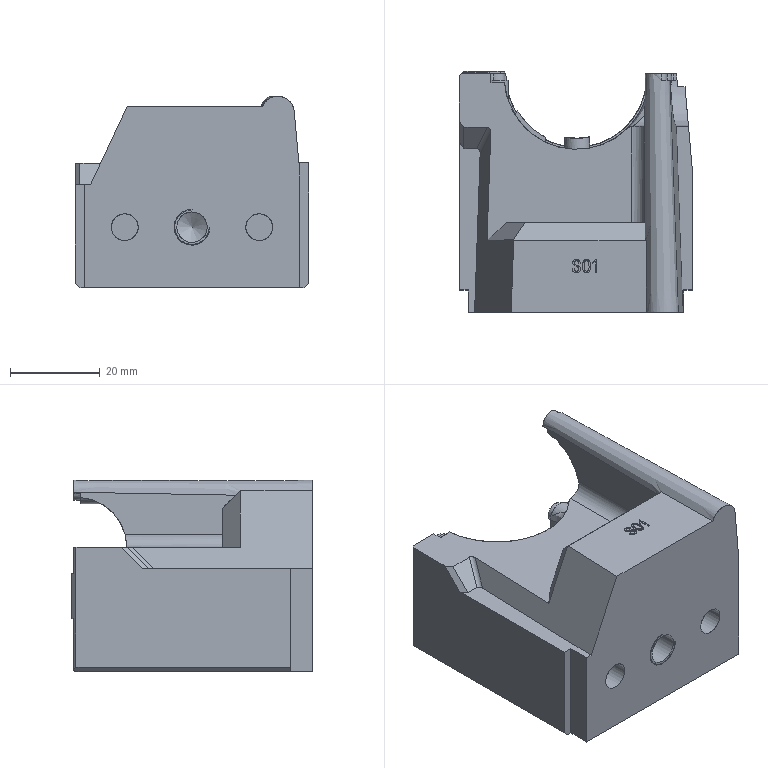NC program | PowerMill | posted with a generic post | part box 52 x 53.756 x 42.711 mm
Lines 1 to 909 of 52163:
%
O0001
N104 ( POWERMILL CB  : 2026004.0)
N105 ( POST VER      : 2026.0.0.5161)
N106 ( OPTION FILE   : FANUC)
N107 ( OUTPUT WORKPLANE : 2)
N108 (  )
N109 ( TOOL LIST )
N110 (---------------------------------------)
N111 ( NO. | ID        | DIA.| TIP RAD|LENGTH)
N112 (---------------------------------------)
N113 (    1|B13R0.8_1_1|13.0 |  0.8   |116.16)
N114 (---------------------------------------)
N115 (  )
N116 ( NUMBER OF TOOLPATHS: 1.0 )
N117 ( ESTIMATED PROGRAM DURATION: 0 HOURS 17 MIN 51 SEC)
N118 (  )
N119 G00 G21 G80 G40 G17
N120 G90
N121 G54
N122 G53 Z0.0
N123 (---------------)
N124 ( START TOOLPATH : 05开粗-B13R0.8-偏置区域清除 )
N125 (---------------)
N126 ( TOOL NO.    :1 )
N127 ( TOOL TYPE   : TIPRADIUSED)
N128 ( TOOL ID     : B13R0.8_1_1)
N129 ( TOOL DIA    : 13.0 LENGTH 116.16)
N130 T1
N131 M6
N132 S2200 M03
N133 G00 G90 X0.1113 Y-6.4944
N134 G43 Z74.256 H1
N135
N136 G05 P10000 R8
N137 Z57.1261
N138 G01 Z54.1261 F2400.0
N139 X0.1108 Y-6.1369 F4000.0
N140 X0.0999 Y0.7514
N141 X0.0891 Y7.6396
N142 X0.0782 Y14.5279
N143 X0.0675 Y21.3365
N144 X4.0078 Y21.3427
N145 G03 X4.3816 Y21.7172 I-0.0006 J0.3745
N146 G01 Y21.9928
N147 G03 X4.0078 Y22.3673 I-0.3744 J0.0
N148 G01 X-3.8728 Y22.3797
N149 G03 X-4.2726 Y21.9805 I-0.0006 J-0.3992
N150 G01 Y21.7295
N151 G03 X-3.8728 Y21.3303 I0.3992 J0.0
N152 G01 X0.0675 Y21.3365
N153 X0.0782 Y14.5279
N154 X9.1921
N155 G03 X11.4721 Y16.8079 I0.0 J2.28
N156 G01 Y26.9021
N157 G03 X9.1921 Y29.1821 I-2.28 J0.0
N158 G01 X-9.1921
N159 G03 X-11.4721 Y26.9021 I0.0 J-2.28
N160 G01 Y16.8079
N161 G03 X-9.1921 Y14.5279 I2.28 J0.0
N162 G01 X0.0782
N163 X0.0891 Y7.6396
N164 X16.0804
N165 G03 X18.3604 Y9.9196 I0.0 J2.28
N166 G01 Y33.7904
N167 G03 X16.0804 Y36.0704 I-2.28 J0.0
N168 G01 X-16.0804
N169 G03 X-18.3604 Y33.7904 I0.0 J-2.28
N170 G01 Y9.9196
N171 G03 X-16.0804 Y7.6396 I2.28 J0.0
N172 G01 X0.0891
N173 X0.0999 Y0.7514
N174 X22.9686
N175 G03 X25.2486 Y3.0314 I0.0 J2.28
N176 G01 Y40.6786
N177 G03 X22.9686 Y42.9586 I-2.28 J0.0
N178 G01 X-22.9686
N179 G03 X-25.2486 Y40.6786 I0.0 J-2.28
N180 G01 Y3.0314
N181 G03 X-22.9686 Y0.7514 I2.28 J0.0
N182 G01 X0.0999
N183 X0.1108 Y-6.1369
N184 G00 Z61.9962
N185 G01 X0.5356 Y-6.6475 F10000.0
N186 G00 Z56.9962
N187 G01 Z53.9962 F2400.0
N188 X0.5308 Y-6.29 F4000.0
N189 X0.4383 Y0.5982
N190 X0.3457 Y7.4865
N191 X0.2532 Y14.3747
N192 X0.163 Y21.0963
N193 X3.9444 Y21.1471
N194 G03 X4.4379 Y21.6279 I-0.0067 J0.5006
N195 G01 X4.4559 Y22.0838
N196 G03 X3.8937 Y22.6684 I-0.5619 J0.0222
N197 G01 X-3.6277 Y22.6646
N198 G03 X-4.2926 Y21.9993 I0.0003 J-0.6653
N199 G01 Y21.7107
N200 G03 X-3.6184 Y21.0455 I0.6652 J0.0
N201 G01 X0.163 Y21.0963
N202 X0.2532 Y14.3747
N203 X9.3453
N204 G03 X11.6253 Y16.6547 I0.0 J2.28
N205 G01 Y27.0553
N206 G03 X9.3453 Y29.3353 I-2.28 J0.0
N207 G01 X-9.3453
N208 G03 X-11.6253 Y27.0553 I0.0 J-2.28
N209 G01 Y16.6547
N210 G03 X-9.3453 Y14.3747 I2.28 J0.0
N211 G01 X0.2532
N212 X0.3457 Y7.4865
N213 X16.2335
N214 G03 X18.5135 Y9.7665 I0.0 J2.28
N215 G01 Y33.9435
N216 G03 X16.2335 Y36.2235 I-2.28 J0.0
N217 G01 X-16.2335
N218 G03 X-18.5135 Y33.9435 I0.0 J-2.28
N219 G01 Y9.7665
N220 G03 X-16.2335 Y7.4865 I2.28 J0.0
N221 G01 X0.3457
N222 X0.4383 Y0.5982
N223 X23.1218
N224 G03 X25.4018 Y2.8782 I0.0 J2.28
N225 G01 Y40.8318
N226 G03 X23.1218 Y43.1118 I-2.28 J0.0
N227 G01 X-23.1218
N228 G03 X-25.4018 Y40.8318 I0.0 J-2.28
N229 G01 Y2.8782
N230 G03 X-23.1218 Y0.5982 I2.28 J0.0
N231 G01 X0.4383
N232 X0.5308 Y-6.29
N233 G00 Z61.8662
N234 G01 X32.7442 Y19.9801 F10000.0
N235 G00 Z56.8662
N236 G01 Z53.8662 F2400.0
N237 X32.3867 Y19.9723 F4000.0
N238 X31.0673 Y19.9436
N239 X31.0701 Y19.8162
N240 X31.0601 Y19.3065
N241 X31.0666 Y18.7968
N242 X31.0653 Y16.758
N243 X31.0571 Y16.2483
N244 X31.0695 Y14.7192
N245 X31.0572 Y14.2095
N246 X31.0691 Y13.6998
N247 X31.0589 Y12.6804
N248 X31.0703 Y12.1707
N249 X31.0534 Y11.661
N250 X31.0203 Y11.1513
N251 X30.9333 Y10.6416
N252 X30.8369 Y10.2018
N253 X30.6364 Y9.6222
N254 X30.4029 Y9.1125
N255 X30.3272 Y8.9646
N256 X30.1081 Y8.6028
N257 X29.8175 Y8.1763
N258 X29.2897 Y7.5834
N259 X28.7136 Y7.0737
N260 X28.2884 Y6.7693
N261 X27.9485 Y6.564
N262 X27.269 Y6.2396
N263 X26.8552 Y6.1018
N264 X26.7954 Y6.0798
N265 X26.7371 Y6.0543
N266 X26.2496 Y5.938
N267 X25.7399 Y5.8564
N268 X25.2302 Y5.8153
N269 X24.7205 Y5.8115
N270 X20.1332
N271 X19.6235 Y5.8132
N272 X19.1138 Y5.8419
N273 X18.6041 Y5.9218
N274 X18.0299 Y6.0543
N275 X17.5847 Y6.2167
N276 X17.075 Y6.44
N277 X16.8238 Y6.564
N278 X16.5653 Y6.7223
N279 X16.0556 Y7.0752
N280 X15.5459 Y7.5088
N281 X15.5246 Y7.5317
N282 X15.4787 Y7.5781
N283 X15.43 Y7.6215
N284 X15.3271 Y7.7343
N285 G03 X14.8463 Y8.0329 I-0.7684 J-0.7008
N286 G01 X14.6372 Y8.0931
N287 X14.0168 Y8.3401
N288 X13.5071 Y8.6065
N289 X12.9974 Y8.9155
N290 X12.71 Y9.1125
N291 X12.4877 Y9.2889
N292 X12.1032 Y9.6222
N293 X11.978 Y9.7414
N294 X11.4683 Y10.3005
N295 X11.1999 Y10.6416
N296 X10.9586 Y10.9981
N297 X10.5963 Y11.661
N298 X10.4489 Y11.9594
N299 X10.1897 Y12.6804
N300 X10.0531 Y13.1901
N301 X9.9392 Y13.7254
N302 X9.8915 Y14.2095
N303 X9.8693 Y14.7192
N304 X9.8702 Y15.7386
N305 X9.8593 Y16.2483
N306 X9.8679 Y16.758
N307 X9.8683 Y18.7968
N308 X9.8771 Y19.1808
N309 X3.9411 Y20.1683
N310 X-1.8594 Y21.1332
N311 X-8.2402 Y22.1947
N312 G02 X-6.8631 Y27.6617 I33.987 J-5.654
N313 G01 X-6.5703 Y28.5203
N314 G03 X-9.1795 Y31.4912 I-2.1579 J0.736
N315 G01 X-11.4482 Y31.033
N316 G03 X-13.2769 Y28.8083 I0.4513 J-2.2348
N317 G01 X-13.3393 Y14.7947
N318 G03 X-9.5029 Y13.1184 I2.28 J-0.0102
N319 G01 X-9.4326 Y13.184
N320 G03 X-8.709 Y14.8478 I-1.5564 J1.6661
N321 G01 X-8.7072 Y16.5763
N322 G02 X-8.2402 Y22.1947 I34.4541 J-0.0356
N323 G01 X-1.8594 Y21.1332
N324 G02 X7.3267 Y35.3016 I19.8002 J-2.7754
N325 G01 X7.8854 Y35.6516
N326 G03 X7.1291 Y38.2188 I-0.7378 J1.1777
N327 G01 X-17.9262 Y37.8857
N328 G03 X-20.1759 Y35.6059 I0.0303 J-2.2798
N329 G01 X-20.1754 Y8.0997
N330 G03 X-17.9475 Y5.8203 I2.28 J0.0
N331 G01 X-3.0171 Y5.479
N332 G03 X-0.8666 Y8.1726 I0.0495 J2.1657
N333 G01 X-1.4308 Y10.4184
N334 G02 X-1.9216 Y13.928 I16.0882 J4.0393
N335 G01 X-2.0428 Y17.7194
N336 G02 X-1.8594 Y21.1332 I19.9836 J0.6384
N337 G01 X3.9411 Y20.1683
N338 G03 X3.8616 Y18.5751 I13.0595 J-1.45
N339 G01 X3.9036 Y14.7254
N340 X3.9107 Y14.3953
N341 X3.9269 Y13.9974
N342 G03 X4.2304 Y11.8821 I10.7305 J0.4603
N343 G01 X4.3476 Y11.4149
N344 G03 X5.4674 Y8.5923 I11.4481 J2.9086
N345 G01 X5.653 Y8.2579
N346 G03 X7.2915 Y6.0191 I9.713 J5.3897
N347 G01 X7.6054 Y5.6869
N348 G03 X8.5223 Y4.8299 I7.3408 J6.9354
N349 G01 X8.656 Y4.7197
N350 G03 X10.4097 Y3.5012 I8.2714 J10.0333
N351 G01 X11.833 Y2.6757
N352 X13.2605 Y1.7466
N353 G03 X14.554 Y1.0341 I5.4508 J8.3652
N354 G01 X14.9156 Y0.8699
N355 X15.2718 Y0.7169
N356 G03 X17.0407 Y0.1532 I3.874 J9.1004
N357 G01 X17.1905 Y0.1206
N358 G03 X19.7362 Y-0.1529 I2.5407 J11.6639
N359 G01 X25.2718 Y-0.1506
N360 X26.108 Y-0.1454
N361 G02 X26.2332 Y-0.2694 I0.0008 J-0.1244
N362 G02 X26.1087 Y-0.3942 I-0.1244 J-0.0004
N363 G01 X-25.9103 Y-0.3625
N364 G02 X-26.1927 Y-0.2454 I0.0003 J0.3998
N365 G01 X-26.2454 Y-0.1927
N366 G02 X-26.3625 Y0.09 I0.2827 J0.2827
N367 G01 Y43.62
N368 G02 X-26.2454 Y43.9027 I0.3998 J0.0
N369 G01 X-26.1927 Y43.9554
N370 G02 X-25.91 Y44.0725 I0.2827 J-0.2827
N371 G01 X25.91
N372 G02 X26.1927 Y43.9554 I0.0 J-0.3998
N373 G01 X26.2454 Y43.9027
N374 G02 X26.3625 Y43.6225 I-0.2827 J-0.2827
N375 G01 X26.4201 Y34.2515
N376 G02 X26.0553 Y33.9091 I-0.3411 J-0.0021
N377 G01 X25.4687 Y33.9499
N378 G03 X22.2599 Y34.0498 I-2.9097 J-41.8508
N379 G01 X20.0669 Y34.0342
N380 G03 X16.3646 Y33.467 I0.0924 J-12.9697
N381 G01 X16.1848 Y33.412
N382 G03 X12.3027 Y31.4185 I3.616 J-11.8184
N383 G01 X11.4881 Y30.7968
N384 X11.3847 Y30.7224
N385 X9.9321 Y29.7933
N386 X9.5002 Y29.5042
N387 G03 X8.5419 Y28.7763 I5.7709 J-8.5926
N388 G01 X8.3255 Y28.5911
N389 G03 X7.4666 Y27.7624 I6.4971 J-7.5934
N390 G01 X7.3288 Y27.6126
N391 G03 X3.9411 Y20.1683 I9.6718 J-8.8943
N392 G01 X9.8771 Y19.1808
N393 X9.88 Y19.3065
N394 X9.9392 Y19.8562
N395 X10.0303 Y20.3259
N396 X10.1698 Y20.8356
N397 X10.3331 Y21.3453
N398 X10.4489 Y21.6232
N399 X10.5554 Y21.855
N400 X10.8257 Y22.3647
N401 X10.9586 Y22.5886
N402 X11.1544 Y22.8744
N403 X11.4683 Y23.2881
N404 X12.0232 Y23.8938
N405 X12.4877 Y24.2985
N406 X12.6189 Y24.4035
N407 X12.9974 Y24.6692
N408 X13.3778 Y24.9132
N409 X14.0168 Y25.2453
N410 X14.5365 Y25.4568
N411 X14.6546 Y25.4958
N412 G03 X15.1193 Y25.8078 I-0.326 J0.9876
N413 G01 X15.226 Y25.9326
N414 X15.5459 Y26.2736
N415 X15.723 Y26.4423
N416 X16.0556 Y26.7163
N417 X16.3821 Y26.952
N418 X17.075 Y27.3524
N419 X17.3042 Y27.4617
N420 X18.0944 Y27.748
N421 X18.6041 Y27.8672
N422 X19.1138 Y27.9454
N423 X19.3529 Y27.9714
N424 X19.6235 Y27.9819
N425 X24.7205 Y27.9821
N426 X25.4189 Y27.9714
N427 X26.2496 Y27.8512
N428 X26.7593 Y27.7251
N429 X27.464 Y27.4617
N430 X27.7787 Y27.3108
N431 X28.3822 Y26.952
N432 X28.7981 Y26.6463
N433 X29.0354 Y26.4423
N434 X29.3078 Y26.1823
N435 X29.5456 Y25.9326
N436 X29.8175 Y25.6041
N437 X29.9431 Y25.4229
N438 X30.3272 Y24.8239
N439 X30.5253 Y24.4035
N440 X30.7363 Y23.8938
N441 X30.8369 Y23.582
N442 X30.9878 Y22.8744
N443 X31.04 Y22.3647
N444 X31.0584 Y21.855
N445 X31.059 Y20.3259
N446 X31.0673 Y19.9436
N447 X32.3867 Y19.9723
N448 G00 Z61.9056
N449 G01 X21.2873 Y27.9969 F10000.0
N450 G00 Z56.9056
N451 G01 Z53.9056 F2400.0
N452 Y27.9919 F4000.0
N453 X21.7512 Y21.0925
N454 G03 X20.6948 Y20.7504 I0.1529 J-2.2749
N455 G01 X18.1033 Y19.1289
N456 G03 X17.0326 Y17.1917 I1.2093 J-1.9328
N457 G01 X17.0341 Y16.4323
N458 G03 X18.1924 Y14.4518 I2.28 J0.0045
N459 G01 X20.7813 Y12.9888
N460 G03 X24.183 Y14.9732 I1.1217 J1.985
N461 G01 X24.1841 Y18.8169
N462 G03 X21.7512 Y21.0925 I-2.28 J0.0007
N463 G01 X21.2873 Y27.9919
N464 G00 Z61.7363
N465 G01 X32.8067 Y16.757 F10000.0
N466 G00 Z56.7363
N467 G01 Z53.7363 F2400.0
N468 X32.4492 Y16.7572 F4000.0
N469 X31.3392 Y16.758
N470 X31.3374 Y14.2095
N471 X31.3311 Y11.661
N472 X31.2937 Y11.1513
N473 X31.2139 Y10.6416
N474 X31.0984 Y10.1319
N475 X30.9243 Y9.6222
N476 X30.8369 Y9.3936
N477 X30.7046 Y9.1125
N478 X30.43 Y8.6028
N479 X30.3272 Y8.4346
N480 X30.0876 Y8.0931
N481 X29.8175 Y7.7507
N482 X29.668 Y7.5834
N483 X29.3078 Y7.2185
N484 X29.1442 Y7.0737
N485 X28.7981 Y6.7934
N486 X28.4716 Y6.564
N487 X28.2884 Y6.4484
N488 X27.7787 Y6.1714
N489 X27.5282 Y6.0543
N490 X27.269 Y5.9492
N491 X26.7593 Y5.782
N492 X26.2496 Y5.6558
N493 X25.7399 Y5.5773
N494 X25.4548 Y5.5446
N495 X24.7205 Y5.5338
N496 X20.1332
N497 X19.6235 Y5.5354
N498 X19.3199 Y5.5446
N499 X19.1138 Y5.5639
N500 X18.6041 Y5.6398
N501 X18.0944 Y5.76
N502 X17.5847 Y5.9212
N503 X17.2408 Y6.0543
N504 X17.075 Y6.1335
N505 X16.5653 Y6.4
N506 X16.2982 Y6.564
N507 X16.0556 Y6.7331
N508 X15.6185 Y7.0737
N509 X15.1574 Y7.5247
N510 G03 X14.766 Y7.7655 I-0.7272 J-0.7435
N511 G01 X14.5265 Y7.8472
N512 X14.0168 Y8.0428
N513 X13.5071 Y8.2916
N514 X12.9675 Y8.6028
N515 X12.4877 Y8.9423
N516 X12.2743 Y9.1125
N517 X11.978 Y9.368
N518 X11.7107 Y9.6222
N519 X11.4683 Y9.8809
N520 X11.2568 Y10.1319
N521 X10.9586 Y10.5119
N522 X10.8701 Y10.6416
N523 X10.4489 Y11.3343
N524 X10.2902 Y11.661
N525 X10.0742 Y12.1707
N526 X9.9392 Y12.5426
N527 X9.7691 Y13.1901
N528 X9.6721 Y13.6998
N529 X9.6179 Y14.2095
N530 X9.5919 Y14.7192
N531 X9.5916 Y16.4959
N532 X3.6811 Y16.832
N533 X-2.2487 Y17.1693
N534 X-8.7133 Y17.537
N535 X-8.649 Y18.6666
N536 G02 X-6.8964 Y26.981 I28.2091 J-1.6045
N537 G01 X-6.1734 Y28.9093
N538 G03 X-8.624 Y31.9203 I-2.1053 J0.7893
N539 G01 X-11.7367 Y31.4367
N540 G03 X-13.6667 Y29.1818 I0.35 J-2.253
N541 G01 X-13.6545 Y14.4205
N542 G03 X-12.7459 Y12.6009 I2.28 J0.0019
N543 G01 X-12.5537 Y12.4562
N544 G03 X-8.906 Y14.1482 I1.3714 J1.8215
N545 G01 X-8.7133 Y17.537
N546 X-2.2487 Y17.1693
N547 G02 X8.3111 Y35.7463 I21.8088 J-0.1072
N548 G01 X8.8989 Y36.1002
N549 G03 X8.185 Y38.6087 I-0.6969 J1.1575
N550 G01 X-18.3144 Y38.2755
N551 G03 X-20.5657 Y35.9954 I0.0287 J-2.2798
N552 G01 X-20.5623 Y7.6865
N553 G03 X-18.3401 Y5.4075 I2.28 J0.0003
N554 G01 X-2.4995 Y5.0058
N555 G03 X-0.4778 Y7.7379 I0.0527 J2.0751
N556 G01 X-1.0742 Y9.5252
N557 G02 X-2.0397 Y13.9499 I20.0702 J6.6972
N558 G01 X-2.1228 Y14.7197
N559 G02 X-2.2487 Y17.1693 I21.6829 J2.3424
N560 G01 X3.6811 Y16.832
N561 X3.68 Y16.29
N562 G03 X12.1494 Y2.4703 I15.4623 J-0.0291
N563 G01 X13.8572 Y1.6043
N564 G03 X24.0007 Y-0.2791 I8.2776 J16.3241
N565 G01 X25.9908 Y-0.0752
N566 G02 X26.4842 Y-0.4992 I0.0457 J-0.4459
N567 G02 X26.0346 Y-0.9694 I-0.4477 J-0.0219
N568 G01 X-25.653 Y-0.7523
N569 G02 X-26.284 Y-0.4894 I0.0038 J0.8976
N570 G01 X-26.4894 Y-0.284
N571 G02 X-26.7523 Y0.3508 I0.6347 J0.6348
N572 G01 Y43.3592
N573 G02 X-26.4894 Y43.994 I0.8976 J0.0001
N574 G01 X-26.284 Y44.1994
N575 G02 X-25.6492 Y44.4623 I0.6348 J-0.6347
N576 G01 X25.6492
N577 G02 X26.284 Y44.1994 I0.0 J-0.8976
N578 G01 X26.4894 Y43.994
N579 G02 X26.752 Y43.3837 I-0.6347 J-0.6347
N580 G01 X26.9761 Y35.1461
N581 G02 X25.3241 Y33.7397 I-1.3924 J-0.0379
N582 G01 X24.9169 Y33.817
N583 G03 X12.7268 Y31.5194 I-3.1664 J-16.6872
N584 G01 X10.8498 Y30.3424
N585 G03 X3.6822 Y17.4159 I8.1243 J-12.9553
N586 G01 X3.6811 Y16.832
N587 X9.5916 Y16.4959
N588 X9.5911 Y18.7968
N589 X9.6079 Y19.3065
N590 X9.6601 Y19.8162
N591 X9.7521 Y20.3259
N592 X9.9392 Y21.0439
N593 X10.0444 Y21.3453
N594 X10.2554 Y21.855
N595 X10.4489 Y22.246
N596 X10.8239 Y22.8744
N597 X10.9586 Y23.0733
N598 X11.1966 Y23.3841
N599 X11.6437 Y23.8938
N600 X11.978 Y24.2202
N601 X12.4877 Y24.6474
N602 X12.8635 Y24.9132
N603 X13.5071 Y25.295
N604 X13.7545 Y25.4229
N605 X14.0168 Y25.5398
N606 X14.5265 Y25.7385
N607 G03 X14.9581 Y26.0443 I-0.3656 J0.9737
N608 G01 X15.0362 Y26.1375
N609 X15.3319 Y26.4423
N610 X15.5459 Y26.6441
N611 X15.9181 Y26.952
N612 X16.0556 Y27.0534
N613 X16.6977 Y27.4617
N614 X17.075 Y27.6565
N615 X17.5847 Y27.8629
N616 X17.8895 Y27.9714
N617 X18.0944 Y28.0259
N618 X18.6041 Y28.142
N619 X19.1138 Y28.2155
N620 X19.6235 Y28.2489
N621 X24.7205 Y28.25
N622 X25.2302 Y28.2449
N623 X25.7399 Y28.2061
N624 X26.2496 Y28.1259
N625 X26.8784 Y27.9714
N626 X27.269 Y27.8347
N627 X27.7787 Y27.6137
N628 X28.0709 Y27.4617
N629 X28.2884 Y27.3312
N630 X28.7981 Y26.9884
N631 X29.3078 Y26.5658
N632 X29.4371 Y26.4423
N633 X29.8175 Y26.035
N634 X29.9004 Y25.9326
N635 X30.3272 Y25.3531
N636 X30.5809 Y24.9132
N637 X30.8369 Y24.392
N638 X31.022 Y23.8938
N639 X31.1688 Y23.3841
N640 X31.2654 Y22.8744
N641 X31.3189 Y22.3647
N642 X31.3398 Y21.855
N643 X31.3346 Y21.3453
N644 X31.3409 Y19.3065
N645 X31.3392 Y16.758
N646 X32.4492 Y16.7572
N647 G00 Z61.6064
N648 G01 X32.8432 Y16.7574 F10000.0
N649 G00 Z56.6064
N650 G01 Z53.6064 F2400.0
N651 X32.4857 Y16.7576 F4000.0
N652 X31.4906 Y16.758
N653 X31.4885 Y11.661
N654 X31.4526 Y11.1513
N655 X31.3752 Y10.6416
N656 X31.2569 Y10.1319
N657 X31.0915 Y9.6222
N658 X30.8777 Y9.1125
N659 X30.6099 Y8.6028
N660 X30.3272 Y8.1598
N661 X29.876 Y7.5834
N662 X29.3078 Y7.0129
N663 X28.7981 Y6.6082
N664 X28.2884 Y6.2761
N665 X27.7787 Y6.0037
N666 X27.269 Y5.79
N667 X26.7593 Y5.6209
N668 X26.4611 Y5.5446
N669 X26.2496 Y5.5026
N670 X25.7399 Y5.4225
N671 X25.2302 Y5.3843
N672 X24.7205 Y5.3809
N673 X20.1332
N674 X19.6235 Y5.3826
N675 X19.1138 Y5.4143
N676 X18.6041 Y5.4866
N677 X18.3072 Y5.5446
N678 X18.0944 Y5.5984
N679 X17.5847 Y5.7569
N680 X17.075 Y5.9627
N681 X16.5653 Y6.2228
N682 X16.0556 Y6.5431
N683 X15.5459 Y6.9399
N684 X15.3954 Y7.0737
N685 X15.0689 Y7.3955
N686 G03 X14.6513 Y7.6468 I-0.7301 J-0.7406
N687 G01 X14.5265 Y7.6861
N688 X14.0168 Y7.8811
N689 X13.5071 Y8.1165
N690 X12.9974 Y8.4063
N691 X12.6932 Y8.6028
N692 X12.4877 Y8.7496
N693 X12.0386 Y9.1125
N694 X11.5014 Y9.6222
N695 X11.0588 Y10.1319
N696 X10.9586 Y10.259
N697 X10.6869 Y10.6416
N698 X10.4489 Y11.0274
N699 X10.1192 Y11.661
N700 X9.9392 Y12.0879
N701 X9.7396 Y12.6804
N702 X9.6111 Y13.1901
N703 X9.5176 Y13.6998
N704 X9.4622 Y14.2095
N705 X9.4419 Y14.7192
N706 X9.4415 Y18.7968
N707 X9.4578 Y19.3065
N708 X9.4618 Y19.3457
N709 X3.8515 Y20.5297
N710 X-1.8715 Y21.7374
N711 X-8.1835 Y23.0695
N712 G02 X-6.695 Y28.0832 I31.7817 J-6.7071
N713 G01 X-6.3767 Y28.906
N714 G03 X-8.8496 Y31.9517 I-2.1077 J0.8155
N715 G01 X-11.7911 Y31.47
N716 G03 X-13.7026 Y29.2183 I0.3685 J-2.25
N717 G01 X-13.6915 Y14.3949
N718 G03 X-13.1019 Y12.8665 I2.28 J0.0017
N719 G01 X-12.9897 Y12.7427
N720 G03 X-9.0219 Y14.1661 I1.6903 J1.5301
N721 G01 X-8.8479 Y17.8818
N722 G02 X-8.1835 Y23.0695 I32.4459 J-1.5194
N723 G01 X-1.8715 Y21.7374
N724 G02 X8.1132 Y35.7623 I20.6705 J-4.1492
N725 G01 X8.6954 Y36.1046
N726 G03 X7.9868 Y38.6446 I-0.6914 J1.1759
N727 G01 X-18.3504 Y38.3114
N728 G03 X-20.6016 Y36.0314 I0.0288 J-2.2798
N729 G01 X-20.5989 Y7.6566
N730 G03 X-18.3751 Y5.3775 I2.28 J0.0002
N731 G01 X-2.7284 Y4.9917
N732 G03 X-0.6886 Y7.7198 I0.0515 J2.0881
N733 G01 X-1.2663 Y9.5146
N734 G02 X-2.2506 Y15.4555 I19.54 J6.2894
N735 G01 X-2.2808 Y17.2302
N736 G02 X-1.8715 Y21.7374 I21.0798 J0.358
N737 G01 X3.8515 Y20.5297
N738 G03 X3.5684 Y17.4253 I14.9186 J-2.9257
N739 G01 X3.589 Y15.6717
N740 G03 X11.0667 Y2.9588 I14.842 J0.1744
N741 G01 X13.1735 Y1.7549
N742 G03 X22.8269 Y-0.4318 I8.4071 J14.7122
N743 G01 X26.0708 Y-0.1926
N744 G02 X26.482 Y-0.5614 I0.0282 J-0.3822
N745 G02 X26.0977 Y-0.9581 I-0.383 J-0.0134
N746 G01 X-25.722 Y-0.7882
N747 G02 X-26.3587 Y-0.5232 I0.0029 J0.9046
N748 G01 X-26.5232 Y-0.3587
N749 G02 X-26.7882 Y0.281 I0.6396 J0.6397
N750 G01 Y43.4291
N751 G02 X-26.5232 Y44.0687 I0.9046 J-0.0001
N752 G01 X-26.3587 Y44.2332
N753 G02 X-25.719 Y44.4982 I0.6396 J-0.6396
N754 G01 X25.719
N755 G02 X26.3587 Y44.2332 I0.0001 J-0.9046
N756 G01 X26.5232 Y44.0687
N757 G02 X26.788 Y43.4483 I-0.6396 J-0.6396
N758 G01 X26.9676 Y35.0221
N759 G02 X25.7303 Y33.8909 I-1.1141 J-0.0237
N760 G01 X23.3492 Y34.1557
N761 G03 X12.7205 Y31.7456 I-1.8387 J-16.5333
N762 G01 X10.7369 Y30.5111
N763 G03 X3.8515 Y20.5297 I8.0332 J-12.9071
N764 G01 X9.4618 Y19.3457
N765 X9.5092 Y19.8162
N766 X9.5953 Y20.3259
N767 X9.7225 Y20.8356
N768 X9.9392 Y21.4941
N769 X10.092 Y21.855
N770 X10.3438 Y22.3647
N771 X10.4489 Y22.5539
N772 X10.6426 Y22.8744
N773 X10.9586 Y23.3223
N774 X11.435 Y23.8938
N775 X11.9559 Y24.4035
N776 X12.5954 Y24.9132
N777 X12.9974 Y25.1788
N778 X13.4219 Y25.4229
N779 X14.0168 Y25.702
N780 X14.4388 Y25.8651
N781 G03 X14.8355 Y26.1377 I-0.3748 J0.9701
N782 G01 X15.1146 Y26.4423
N783 X15.5459 Y26.842
N784 X15.6753 Y26.952
N785 X16.0556 Y27.236
N786 X16.3973 Y27.4617
N787 X16.5653 Y27.5597
N788 X17.075 Y27.8198
N789 X17.4285 Y27.9714
N790 X18.0944 Y28.1848
N791 X18.6041 Y28.2961
N792 X19.1138 Y28.3688
N793 X19.6235 Y28.3999
N794 X20.1332 Y28.403
N795 X24.7205
N796 X25.2302 Y28.3974
N797 X25.7399 Y28.3588
N798 X26.2496 Y28.2799
N799 X26.7593 Y28.1618
N800 X27.3348 Y27.9714
N801 X27.7787 Y27.7802
N802 X28.3698 Y27.4617
N803 X28.7981 Y27.1744
N804 X29.0932 Y26.952
N805 X29.3078 Y26.768
N806 X29.6489 Y26.4423
N807 X29.8175 Y26.2623
N808 X30.0946 Y25.9326
N809 X30.3272 Y25.623
N810 X30.4587 Y25.4229
N811 X30.7537 Y24.9132
N812 X30.8369 Y24.7557
N813 X30.9932 Y24.4035
N814 X31.1824 Y23.8938
N815 X31.324 Y23.3841
N816 X31.4213 Y22.8744
N817 X31.476 Y22.3647
N818 X31.4927 Y21.855
N819 X31.4906 Y16.758
N820 X32.4857 Y16.7576
N821 G00 Z61.4765
N822 G01 X32.8572 Y17.0128 F10000.0
N823 G00 Z56.4765
N824 G01 Z53.4765 F2400.0
N825 X32.4997 F4000.0
N826 X31.6227
N827 Y12.1707
N828 X31.6204 Y11.661
N829 X31.5872 Y11.1513
N830 X31.5129 Y10.6416
N831 X31.3963 Y10.1319
N832 X31.2349 Y9.6222
N833 X31.025 Y9.1125
N834 X30.7611 Y8.6028
N835 X30.4356 Y8.0931
N836 X30.3272 Y7.9443
N837 X30.0363 Y7.5834
N838 X29.8175 Y7.343
N839 X29.5446 Y7.0737
N840 X29.3078 Y6.864
N841 X28.9267 Y6.564
N842 X28.7981 Y6.4731
N843 X28.2884 Y6.1525
N844 X28.1101 Y6.0543
N845 X27.7787 Y5.8918
N846 X27.269 Y5.6795
N847 X26.8624 Y5.5446
N848 X26.2496 Y5.3947
N849 X25.7399 Y5.3183
N850 X25.2302 Y5.2841
N851 X24.7205 Y5.2803
N852 X20.1332
N853 X19.6235 Y5.2818
N854 X19.1138 Y5.3088
N855 X18.6041 Y5.3816
N856 X18.0944 Y5.4933
N857 X17.9029 Y5.5446
N858 X17.5847 Y5.6487
N859 X17.075 Y5.8499
N860 X16.6577 Y6.0543
N861 X16.0556 Y6.4194
N862 X15.8532 Y6.564
N863 X15.5459 Y6.805
N864 X15.2446 Y7.0737
N865 X15.031 Y7.291
N866 G03 X14.6008 Y7.5541 I-0.7416 J-0.7292
N867 G01 X14.5075 Y7.5834
N868 X14.0168 Y7.7693
N869 X13.5071 Y8.0018
N870 X12.9974 Y8.2869
N871 X12.5157 Y8.6028
N872 X11.8796 Y9.1125
N873 X11.4683 Y9.5096
N874 X11.3619 Y9.6222
N875 X10.9586 Y10.0923
N876 X10.5661 Y10.6416
N877 X10.2608 Y11.1513
N878 X10.0083 Y11.661
N879 X9.9392 Y11.8168
N880 X9.8018 Y12.1707
N881 X9.6324 Y12.6804
N882 X9.5047 Y13.1901
N883 X9.4295 Y13.5944
N884 X9.3605 Y14.2095
N885 X9.3387 Y14.7192
N886 X9.3385 Y18.3542
N887 X3.5372 Y18.9131
N888 X-2.2996 Y19.4755
N889 X-8.7415 Y20.0961
N890 G02 X-7.0976 Y27.3381 I29.1435 J-2.8079
N891 G01 X-6.5079 Y28.9517
N892 G03 X-9.0178 Y31.9616 I-2.1275 J0.7774
N893 G01 X-11.8213 Y31.4814
N894 G03 X-13.7163 Y29.2326 I0.385 J-2.2473
N895 G01 X-13.7063 Y14.3917
N896 G03 X-13.6201 Y13.7724 I2.2801 J0.0015
N897 G01 X-13.5872 Y13.6561
N898 G03 X-9.1174 Y14.1406 I2.1939 J0.6208
N899 G01 X-8.8241 Y19.0385
N900 X-8.7876 Y19.5677
N901 X-8.7415 Y20.0961
N902 X-2.2996 Y19.4755
N903 G02 X7.9106 Y35.7462 I20.7645 J-1.6913
N904 G01 X8.4899 Y36.0866
N905 G03 X7.7727 Y38.6581 I-0.6996 J1.1906
N906 G01 X-18.3642 Y38.325
N907 G03 X-20.6151 Y36.045 I0.0291 J-2.2799
N908 G01 X-20.6132 Y7.6489
N909 G03 X-18.3877 Y5.3697 I2.28 J0.0001
N910 G01 X-2.8827 Y4.9989
N911 G03 X-0.8268 Y7.7311 I0.0503 J2.1018
N912 G01 X-1.3946 Y9.5375
N913 G02 X-2.3387 Y15.4268 I19.6103 J6.1642
N914 G01 X-2.3665 Y17.5057
N915 G02 X-2.2996 Y19.4755 I20.8314 J0.2785
N916 G01 X3.5372 Y18.9131
N917 X3.5094 Y18.3877
N918 X3.5003 Y17.8617
N919 X3.5014 Y15.7339
N920 G03 X11.0719 Y2.787 I14.8692 J0.0077
N921 G01 X13.2866 Y1.5392
N922 G03 X22.1518 Y-0.5163 I7.9374 J14.088
N923 G01 X26.1284 Y-0.2877
N924 G02 X26.4659 Y-0.5977 I0.0183 J-0.3188
N925 G02 X26.1459 Y-0.9258 I-0.3192 J-0.0088
N926 G01 X-25.7732 Y-0.8017
N927 G02 X-26.405 Y-0.5391 I0.0021 J0.8965
N928 G01 X-26.5391 Y-0.405
N929 G02 X-26.8017 Y0.2289 I0.6339 J0.6339
N930 G01 Y43.4811
N931 G02 X-26.5391 Y44.115 I0.8965 J0.0
N932 G01 X-26.405 Y44.2491
N933 G02 X-25.7711 Y44.5117 I0.6339 J-0.6339
N934 G01 X25.7711
N935 G02 X26.405 Y44.2491 I0.0 J-0.8965
N936 G01 X26.5391 Y44.115
N937 G02 X26.8016 Y43.4964 I-0.6339 J-0.6339
N938 G01 X26.948 Y34.913
N939 G02 X26.0253 Y34.0378 I-0.8624 J-0.0147
N940 G01 X22.3194 Y34.2978
N941 G03 X12.5355 Y31.7737 I-1.1154 J-15.9009
N942 G01 X10.2552 Y30.296
N943 G03 X3.5372 Y18.9131 I8.0528 J-12.4266
N944 G01 X9.3385 Y18.3542
N945 X9.3384 Y18.7968
N946 X9.3554 Y19.3065
N947 X9.4295 Y19.995
N948 X9.4915 Y20.3259
N949 X9.6148 Y20.8356
N950 X9.778 Y21.3453
N951 X9.9392 Y21.7654
N952 X10.2277 Y22.3647
N953 X10.5206 Y22.8744
N954 X10.8771 Y23.3841
N955 X11.2978 Y23.8938
N956 X11.4683 Y24.0791
N957 X11.8052 Y24.4035
N958 X11.978 Y24.5566
N959 X12.4231 Y24.9132
N960 X12.9974 Y25.2975
N961 X13.5071 Y25.5822
N962 X14.0168 Y25.8169
N963 X14.3158 Y25.9326
N964 X14.3537 Y25.9459
N965 G03 X14.7754 Y26.2239 I-0.3444 J0.9813
N966 G01 X14.9759 Y26.4423
N967 X15.5136 Y26.952
N968 X16.0556 Y27.3634
N969 X16.2018 Y27.4617
N970 X16.5653 Y27.6763
N971 X17.075 Y27.9348
N972 X17.5847 Y28.1348
N973 X18.0944 Y28.2893
N974 X18.6041 Y28.403
N975 X19.1138 Y28.4773
N976 X19.6235 Y28.507
N977 X20.1332 Y28.5043
N978 X25.2302
N979 X25.609 Y28.4811
N980 X26.2496 Y28.3889
N981 X26.7593 Y28.2665
N982 X27.269 Y28.1063
N983 X27.7787 Y27.8955
N984 X28.2884 Y27.6305
N985 X28.5668 Y27.4617
N986 X28.7981 Y27.3058
N987 X29.255 Y26.952
N988 X29.797 Y26.4423
N989 X30.2353 Y25.9326
N990 X30.3272 Y25.8117
N991 X30.595 Y25.4229
N992 X30.8369 Y25.0109
N993 X31.1263 Y24.4035
N994 X31.3132 Y23.8938
N995 X31.4539 Y23.3841
N996 X31.5514 Y22.8744
N997 X31.6071 Y22.3647
N998 X31.6227 Y21.855
N999 Y17.0128
N1000 X32.4997
N1001 G00 Z61.3465
N1002 G01 X-18.6252 Y50.5675 F10000.0
N1003 G00 Z56.3465
N1004 G01 Z53.3465 F2400.0
N1005 X-18.6208 Y50.21 F4000.0
N1006 X-18.6041 Y48.8179